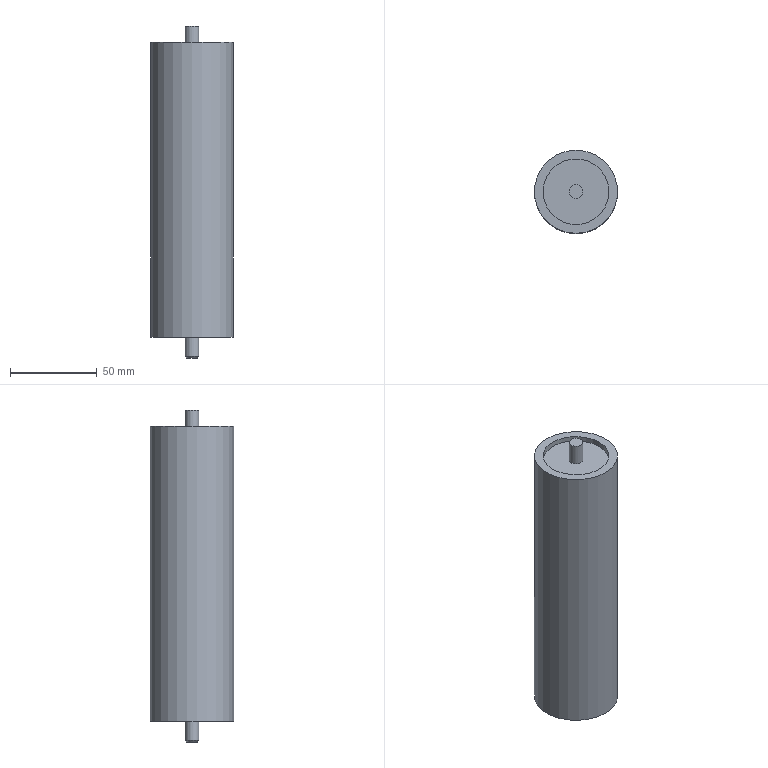Part | STEP file | Idler 3 | 1 solid | 12 faces | box 48.012 x 48.012 x 191.5 mm | volume 302346 mm3 | plane 6 | cylinder 5 | cone 1 | commonest cylinder face diameters 8 x2 38.012 x2 48.012 x1
STEP:
#1=CARTESIAN_POINT('',(0.,-1.398,3.72));
#2=VERTEX_POINT('',#1);
#3=CARTESIAN_POINT('',(0.,-1.24,3.72));
#4=DIRECTION('',(0.,0.,-1.));
#5=DIRECTION('',(0.,1.,0.));
#6=AXIS2_PLACEMENT_3D('',#3,#4,#5);
#7=CIRCLE('',#6,0.1575);
#8=EDGE_CURVE('',#2,#2,#7,.T.);
#9=ORIENTED_EDGE('',*,*,#8,.F.);
#10=EDGE_LOOP('',(#9));
#11=FACE_OUTER_BOUND('',#10,.T.);
#12=CARTESIAN_POINT('',(-0.1969,-2.001,3.72));
#13=DIRECTION('',(0.,0.,-1.));
#14=DIRECTION('',(0.,1.,0.));
#15=AXIS2_PLACEMENT_3D('',#12,#13,#14);
#16=PLANE('',#15);
#17=ADVANCED_FACE('',(#11),#16,.F.);
#18=CARTESIAN_POINT('',(-0.7483,-1.24,-3.346));
#19=VERTEX_POINT('',#18);
#20=CARTESIAN_POINT('',(0.,-1.24,-3.346));
#21=DIRECTION('',(0.,0.,1.));
#22=DIRECTION('',(1.,0.,0.));
#23=AXIS2_PLACEMENT_3D('',#20,#21,#22);
#24=CIRCLE('',#23,0.7483);
#25=EDGE_CURVE('',#19,#19,#24,.T.);
#26=ORIENTED_EDGE('',*,*,#25,.F.);
#27=CARTESIAN_POINT('',(-0.7483,-1.24,-3.228));
#28=VERTEX_POINT('',#27);
#29=CARTESIAN_POINT('',(-0.7483,-1.24,-3.346));
#30=DIRECTION('',(0.,0.,1.));
#31=VECTOR('',#30,0.7483);
#32=LINE('',#29,#31);
#33=EDGE_CURVE('',#19,#28,#32,.T.);
#34=ORIENTED_EDGE('',*,*,#33,.T.);
#35=CARTESIAN_POINT('',(0.,-1.24,-3.228));
#36=DIRECTION('',(0.,0.,-1.));
#37=DIRECTION('',(1.,0.,0.));
#38=AXIS2_PLACEMENT_3D('',#35,#36,#37);
#39=CIRCLE('',#38,0.7483);
#40=EDGE_CURVE('',#28,#28,#39,.T.);
#41=ORIENTED_EDGE('',*,*,#40,.F.);
#42=ORIENTED_EDGE('',*,*,#33,.F.);
#43=EDGE_LOOP('',(#26,#34,#41,#42));
#44=FACE_OUTER_BOUND('',#43,.T.);
#45=CARTESIAN_POINT('',(0.,-1.24,-3.346));
#46=DIRECTION('',(0.,0.,-1.));
#47=DIRECTION('',(1.,0.,0.));
#48=AXIS2_PLACEMENT_3D('',#45,#46,#47);
#49=CYLINDRICAL_SURFACE('',#48,0.7483);
#50=ADVANCED_FACE('',(#44),#49,.F.);
#51=ORIENTED_EDGE('',*,*,#40,.T.);
#52=EDGE_LOOP('',(#51));
#53=FACE_OUTER_BOUND('',#52,.T.);
#54=CARTESIAN_POINT('',(0.,-1.398,-3.228));
#55=VERTEX_POINT('',#54);
#56=CARTESIAN_POINT('',(0.,-1.24,-3.228));
#57=DIRECTION('',(0.,0.,1.));
#58=DIRECTION('',(-1.,0.,0.));
#59=AXIS2_PLACEMENT_3D('',#56,#57,#58);
#60=CIRCLE('',#59,0.1575);
#61=EDGE_CURVE('',#55,#55,#60,.T.);
#62=ORIENTED_EDGE('',*,*,#61,.T.);
#63=EDGE_LOOP('',(#62));
#64=FACE_BOUND('',#63,.T.);
#65=CARTESIAN_POINT('',(0.,-1.24,-3.228));
#66=DIRECTION('',(0.,0.,1.));
#67=DIRECTION('',(1.,0.,0.));
#68=AXIS2_PLACEMENT_3D('',#65,#66,#67);
#69=PLANE('',#68);
#70=ADVANCED_FACE('',(#53,#64),#69,.F.);
#71=CARTESIAN_POINT('',(-0.7483,-1.24,3.346));
#72=VERTEX_POINT('',#71);
#73=CARTESIAN_POINT('',(0.,-1.24,3.346));
#74=DIRECTION('',(0.,0.,-1.));
#75=DIRECTION('',(1.,0.,0.));
#76=AXIS2_PLACEMENT_3D('',#73,#74,#75);
#77=CIRCLE('',#76,0.7483);
#78=EDGE_CURVE('',#72,#72,#77,.T.);
#79=ORIENTED_EDGE('',*,*,#78,.F.);
#80=CARTESIAN_POINT('',(-0.7483,-1.24,3.228));
#81=VERTEX_POINT('',#80);
#82=CARTESIAN_POINT('',(-0.7483,-1.24,3.346));
#83=DIRECTION('',(0.,0.,-1.));
#84=VECTOR('',#83,0.7483);
#85=LINE('',#82,#84);
#86=EDGE_CURVE('',#72,#81,#85,.T.);
#87=ORIENTED_EDGE('',*,*,#86,.T.);
#88=CARTESIAN_POINT('',(0.,-1.24,3.228));
#89=DIRECTION('',(0.,0.,-1.));
#90=DIRECTION('',(1.,0.,0.));
#91=AXIS2_PLACEMENT_3D('',#88,#89,#90);
#92=CIRCLE('',#91,0.7483);
#93=EDGE_CURVE('',#81,#81,#92,.T.);
#94=ORIENTED_EDGE('',*,*,#93,.T.);
#95=ORIENTED_EDGE('',*,*,#86,.F.);
#96=EDGE_LOOP('',(#79,#87,#94,#95));
#97=FACE_OUTER_BOUND('',#96,.T.);
#98=CARTESIAN_POINT('',(0.,-1.24,3.346));
#99=DIRECTION('',(0.,0.,-1.));
#100=DIRECTION('',(1.,0.,0.));
#101=AXIS2_PLACEMENT_3D('',#98,#99,#100);
#102=CYLINDRICAL_SURFACE('',#101,0.7483);
#103=ADVANCED_FACE('',(#97),#102,.F.);
#104=ORIENTED_EDGE('',*,*,#93,.F.);
#105=EDGE_LOOP('',(#104));
#106=FACE_OUTER_BOUND('',#105,.T.);
#107=CARTESIAN_POINT('',(0.,-1.398,3.228));
#108=VERTEX_POINT('',#107);
#109=CARTESIAN_POINT('',(0.,-1.24,3.228));
#110=DIRECTION('',(0.,0.,-1.));
#111=DIRECTION('',(-1.,0.,0.));
#112=AXIS2_PLACEMENT_3D('',#109,#110,#111);
#113=CIRCLE('',#112,0.1575);
#114=EDGE_CURVE('',#108,#108,#113,.T.);
#115=ORIENTED_EDGE('',*,*,#114,.T.);
#116=EDGE_LOOP('',(#115));
#117=FACE_BOUND('',#116,.T.);
#118=CARTESIAN_POINT('',(0.,-1.24,3.228));
#119=DIRECTION('',(0.,0.,1.));
#120=DIRECTION('',(1.,0.,0.));
#121=AXIS2_PLACEMENT_3D('',#118,#119,#120);
#122=PLANE('',#121);
#123=ADVANCED_FACE('',(#106,#117),#122,.T.);
#124=CARTESIAN_POINT('',(0.,-2.185,-3.346));
#125=VERTEX_POINT('',#124);
#126=CARTESIAN_POINT('',(0.,-1.24,-3.346));
#127=DIRECTION('',(0.,0.,1.));
#128=DIRECTION('',(1.,0.,0.));
#129=AXIS2_PLACEMENT_3D('',#126,#127,#128);
#130=CIRCLE('',#129,0.9451);
#131=EDGE_CURVE('',#125,#125,#130,.T.);
#132=ORIENTED_EDGE('',*,*,#131,.F.);
#133=EDGE_LOOP('',(#132));
#134=FACE_OUTER_BOUND('',#133,.T.);
#135=ORIENTED_EDGE('',*,*,#25,.T.);
#136=EDGE_LOOP('',(#135));
#137=FACE_BOUND('',#136,.T.);
#138=CARTESIAN_POINT('',(0.,-0.295,-3.346));
#139=DIRECTION('',(0.,0.,-1.));
#140=DIRECTION('',(-1.,0.,0.));
#141=AXIS2_PLACEMENT_3D('',#138,#139,#140);
#142=PLANE('',#141);
#143=ADVANCED_FACE('',(#134,#137),#142,.T.);
#144=CARTESIAN_POINT('',(0.,-2.185,3.346));
#145=VERTEX_POINT('',#144);
#146=CARTESIAN_POINT('',(0.,-1.24,3.346));
#147=DIRECTION('',(0.,0.,1.));
#148=DIRECTION('',(1.,0.,0.));
#149=AXIS2_PLACEMENT_3D('',#146,#147,#148);
#150=CIRCLE('',#149,0.9451);
#151=EDGE_CURVE('',#145,#145,#150,.T.);
#152=ORIENTED_EDGE('',*,*,#151,.F.);
#153=CARTESIAN_POINT('',(0.,-2.185,0.));
#154=DIRECTION('',(0.,0.,-1.));
#155=VECTOR('',#154,0.9451);
#156=LINE('',#153,#155);
#157=EDGE_CURVE('',#145,#125,#156,.T.);
#158=ORIENTED_EDGE('',*,*,#157,.T.);
#159=ORIENTED_EDGE('',*,*,#131,.T.);
#160=ORIENTED_EDGE('',*,*,#157,.F.);
#161=EDGE_LOOP('',(#152,#158,#159,#160));
#162=FACE_OUTER_BOUND('',#161,.T.);
#163=CARTESIAN_POINT('',(0.,-1.24,0.));
#164=DIRECTION('',(0.,0.,1.));
#165=DIRECTION('',(0.,1.,0.));
#166=AXIS2_PLACEMENT_3D('',#163,#164,#165);
#167=CYLINDRICAL_SURFACE('',#166,0.9451);
#168=ADVANCED_FACE('',(#162),#167,.T.);
#169=ORIENTED_EDGE('',*,*,#151,.T.);
#170=EDGE_LOOP('',(#169));
#171=FACE_OUTER_BOUND('',#170,.T.);
#172=ORIENTED_EDGE('',*,*,#78,.T.);
#173=EDGE_LOOP('',(#172));
#174=FACE_BOUND('',#173,.T.);
#175=CARTESIAN_POINT('',(0.,-1.083,3.346));
#176=DIRECTION('',(0.,0.,1.));
#177=DIRECTION('',(1.,0.,0.));
#178=AXIS2_PLACEMENT_3D('',#175,#176,#177);
#179=PLANE('',#178);
#180=ADVANCED_FACE('',(#171,#174),#179,.T.);
#181=ORIENTED_EDGE('',*,*,#8,.T.);
#182=CARTESIAN_POINT('',(0.,-1.398,3.583));
#183=DIRECTION('',(0.,0.,-1.));
#184=VECTOR('',#183,0.1575);
#185=LINE('',#182,#184);
#186=EDGE_CURVE('',#2,#108,#185,.T.);
#187=ORIENTED_EDGE('',*,*,#186,.T.);
#188=ORIENTED_EDGE('',*,*,#114,.F.);
#189=ORIENTED_EDGE('',*,*,#186,.F.);
#190=EDGE_LOOP('',(#181,#187,#188,#189));
#191=FACE_OUTER_BOUND('',#190,.T.);
#192=CARTESIAN_POINT('',(0.,-1.24,3.583));
#193=DIRECTION('',(0.,0.,1.));
#194=DIRECTION('',(0.,1.,0.));
#195=AXIS2_PLACEMENT_3D('',#192,#193,#194);
#196=CYLINDRICAL_SURFACE('',#195,0.1575);
#197=ADVANCED_FACE('',(#191),#196,.T.);
#198=ORIENTED_EDGE('',*,*,#61,.F.);
#199=CARTESIAN_POINT('',(0.,-1.398,-3.78));
#200=VERTEX_POINT('',#199);
#201=CARTESIAN_POINT('',(0.,-1.398,-3.583));
#202=DIRECTION('',(0.,0.,-1.));
#203=VECTOR('',#202,0.1575);
#204=LINE('',#201,#203);
#205=EDGE_CURVE('',#55,#200,#204,.T.);
#206=ORIENTED_EDGE('',*,*,#205,.T.);
#207=CARTESIAN_POINT('',(0.,-1.083,-3.78));
#208=VERTEX_POINT('',#207);
#209=CARTESIAN_POINT('',(0.,-1.24,-3.78));
#210=DIRECTION('',(0.,0.,-1.));
#211=DIRECTION('',(0.,-1.,0.));
#212=AXIS2_PLACEMENT_3D('',#209,#210,#211);
#213=CIRCLE('',#212,0.1575);
#214=EDGE_CURVE('',#208,#200,#213,.T.);
#215=ORIENTED_EDGE('',*,*,#214,.F.);
#216=CARTESIAN_POINT('',(0.,-1.24,-3.78));
#217=DIRECTION('',(0.,0.,-1.));
#218=DIRECTION('',(0.,-1.,0.));
#219=AXIS2_PLACEMENT_3D('',#216,#217,#218);
#220=CIRCLE('',#219,0.1575);
#221=EDGE_CURVE('',#200,#208,#220,.T.);
#222=ORIENTED_EDGE('',*,*,#221,.F.);
#223=ORIENTED_EDGE('',*,*,#205,.F.);
#224=EDGE_LOOP('',(#198,#206,#215,#222,#223));
#225=FACE_OUTER_BOUND('',#224,.T.);
#226=CARTESIAN_POINT('',(0.,-1.24,-3.583));
#227=DIRECTION('',(0.,0.,1.));
#228=DIRECTION('',(0.,1.,0.));
#229=AXIS2_PLACEMENT_3D('',#226,#227,#228);
#230=CYLINDRICAL_SURFACE('',#229,0.1575);
#231=ADVANCED_FACE('',(#225),#230,.T.);
#232=CARTESIAN_POINT('',(0.,-1.122,-3.819));
#233=VERTEX_POINT('',#232);
#234=CARTESIAN_POINT('',(0.,-1.24,-3.819));
#235=DIRECTION('',(0.,0.,1.));
#236=DIRECTION('',(0.,-1.,0.));
#237=AXIS2_PLACEMENT_3D('',#234,#235,#236);
#238=CIRCLE('',#237,0.1181);
#239=EDGE_CURVE('',#233,#233,#238,.T.);
#240=ORIENTED_EDGE('',*,*,#239,.F.);
#241=EDGE_LOOP('',(#240));
#242=FACE_OUTER_BOUND('',#241,.T.);
#243=CARTESIAN_POINT('',(0.,-1.083,-3.819));
#244=DIRECTION('',(0.,0.,-1.));
#245=DIRECTION('',(-1.,0.,0.));
#246=AXIS2_PLACEMENT_3D('',#243,#244,#245);
#247=PLANE('',#246);
#248=ADVANCED_FACE('',(#242),#247,.T.);
#249=ORIENTED_EDGE('',*,*,#214,.T.);
#250=ORIENTED_EDGE('',*,*,#221,.T.);
#251=CARTESIAN_POINT('',(0.,-1.102,-3.799));
#252=DIRECTION('',(0.,-0.7071,-0.7071));
#253=VECTOR('',#252,0.1378);
#254=LINE('',#251,#253);
#255=EDGE_CURVE('',#208,#233,#254,.T.);
#256=ORIENTED_EDGE('',*,*,#255,.T.);
#257=ORIENTED_EDGE('',*,*,#239,.T.);
#258=ORIENTED_EDGE('',*,*,#255,.F.);
#259=EDGE_LOOP('',(#249,#250,#256,#257,#258));
#260=FACE_OUTER_BOUND('',#259,.T.);
#261=CARTESIAN_POINT('',(0.,-1.24,-3.799));
#262=DIRECTION('',(0.,0.,1.));
#263=DIRECTION('',(0.,-1.,0.));
#264=AXIS2_PLACEMENT_3D('',#261,#262,#263);
#265=CONICAL_SURFACE('',#264,0.1378,0.7854);
#266=ADVANCED_FACE('',(#260),#265,.T.);
#267=CLOSED_SHELL('',(#17,#50,#70,#103,#123,#143,#168,#180,#197,#231,#248,#266));
#268=MANIFOLD_SOLID_BREP('',#267);
#269=(LENGTH_UNIT()NAMED_UNIT(*)SI_UNIT(.MILLI.,.METRE.));
#270=LENGTH_MEASURE_WITH_UNIT(LENGTH_MEASURE(25.4),#269);
#271=DIMENSIONAL_EXPONENTS(1.,0.,0.,0.,0.,0.,0.);
#272=(CONVERSION_BASED_UNIT('inch',#270)LENGTH_UNIT()NAMED_UNIT(#271));
#273=UNCERTAINTY_MEASURE_WITH_UNIT(LENGTH_MEASURE(0.0003937),#272,'','');
#274=(NAMED_UNIT(*)PLANE_ANGLE_UNIT()SI_UNIT($,.RADIAN.));
#275=(NAMED_UNIT(*)SI_UNIT($,.STERADIAN.)SOLID_ANGLE_UNIT());
#276=(GEOMETRIC_REPRESENTATION_CONTEXT(3)GLOBAL_UNCERTAINTY_ASSIGNED_CONTEXT((#273))GLOBAL_UNIT_ASSIGNED_CONTEXT((#272,#274,#275))REPRESENTATION_CONTEXT('',''));
#277=ADVANCED_BREP_SHAPE_REPRESENTATION('',(#268),#276);